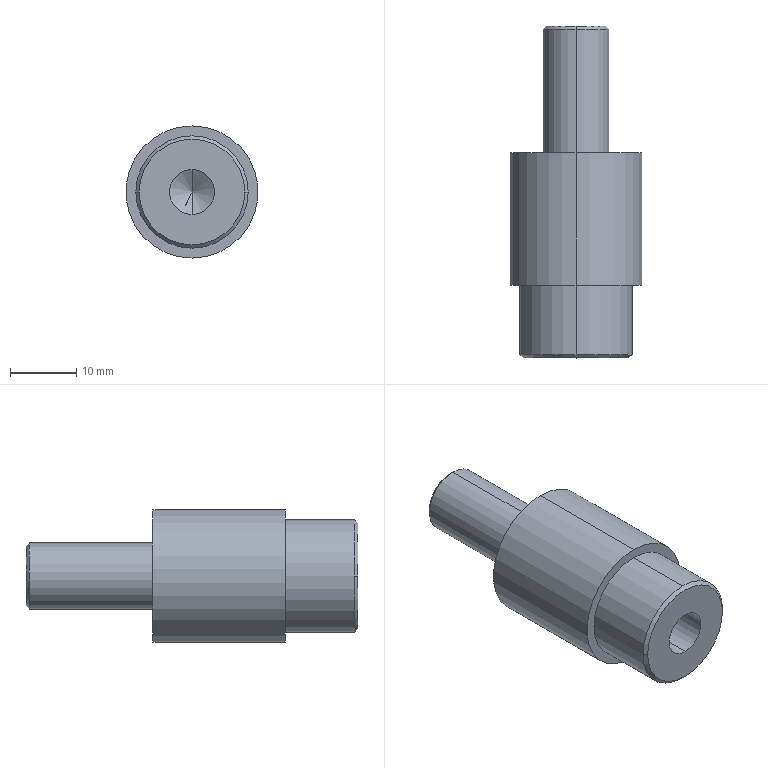Part | SolidWorks | features BaseBody 1 | 1 solid | 18 faces | box 20 x 50.2 x 20 mm | volume 9817 mm3 | cylinder 8 | cone 6 | plane 4 | commonest cylinder face diameters 6.8 x2 10 x2 17 x2 20 x2
STEP:
#1=CARTESIAN_POINT('',(0.,20.,-10.));
#2=VERTEX_POINT('',#1);
#3=CARTESIAN_POINT('',(0.,20.,10.));
#4=VERTEX_POINT('',#3);
#5=CARTESIAN_POINT('',(0.,20.,0.));
#6=DIRECTION('',(0.,-1.,0.));
#7=DIRECTION('',(0.,0.,-1.));
#8=AXIS2_PLACEMENT_3D('',#5,#6,#7);
#9=CIRCLE('',#8,10.);
#10=EDGE_CURVE('',#2,#4,#9,.T.);
#11=ORIENTED_EDGE('',*,*,#10,.T.);
#12=CARTESIAN_POINT('',(0.,0.,10.));
#13=VERTEX_POINT('',#12);
#14=CARTESIAN_POINT('',(0.,20.,10.));
#15=DIRECTION('',(0.,-1.,0.));
#16=VECTOR('',#15,1000.);
#17=LINE('',#14,#16);
#18=EDGE_CURVE('',#4,#13,#17,.T.);
#19=ORIENTED_EDGE('',*,*,#18,.T.);
#20=CARTESIAN_POINT('',(0.,0.,-10.));
#21=VERTEX_POINT('',#20);
#22=CARTESIAN_POINT('',(0.,0.,0.));
#23=DIRECTION('',(0.,1.,0.));
#24=DIRECTION('',(0.,0.,-1.));
#25=AXIS2_PLACEMENT_3D('',#22,#23,#24);
#26=CIRCLE('',#25,10.);
#27=EDGE_CURVE('',#13,#21,#26,.T.);
#28=ORIENTED_EDGE('',*,*,#27,.T.);
#29=CARTESIAN_POINT('',(0.,20.,-10.));
#30=DIRECTION('',(0.,-1.,0.));
#31=VECTOR('',#30,1000.);
#32=LINE('',#29,#31);
#33=EDGE_CURVE('',#2,#21,#32,.T.);
#34=ORIENTED_EDGE('',*,*,#33,.F.);
#35=EDGE_LOOP('',(#11,#19,#28,#34));
#36=FACE_OUTER_BOUND('',#35,.T.);
#37=CARTESIAN_POINT('',(0.,20.,0.));
#38=DIRECTION('',(0.,-1.,0.));
#39=DIRECTION('',(0.,0.,-1.));
#40=AXIS2_PLACEMENT_3D('',#37,#38,#39);
#41=CYLINDRICAL_SURFACE('',#40,10.);
#42=ADVANCED_FACE('',(#36),#41,.T.);
#43=CARTESIAN_POINT('',(8.5,-10.5,0.));
#44=VERTEX_POINT('',#43);
#45=CARTESIAN_POINT('',(0.,-10.5,-8.5));
#46=VERTEX_POINT('',#45);
#47=CARTESIAN_POINT('',(0.,-10.5,0.));
#48=DIRECTION('',(0.,1.,0.));
#49=DIRECTION('',(0.,0.,1.));
#50=AXIS2_PLACEMENT_3D('',#47,#48,#49);
#51=CIRCLE('',#50,8.5);
#52=EDGE_CURVE('',#44,#46,#51,.T.);
#53=ORIENTED_EDGE('',*,*,#52,.T.);
#54=CARTESIAN_POINT('',(0.,0.,-8.5));
#55=VERTEX_POINT('',#54);
#56=CARTESIAN_POINT('',(0.,-11.,-8.5));
#57=DIRECTION('',(0.,1.,0.));
#58=VECTOR('',#57,1000.);
#59=LINE('',#56,#58);
#60=EDGE_CURVE('',#46,#55,#59,.T.);
#61=ORIENTED_EDGE('',*,*,#60,.T.);
#62=CARTESIAN_POINT('',(0.,0.,8.5));
#63=VERTEX_POINT('',#62);
#64=CARTESIAN_POINT('',(0.,0.,0.));
#65=DIRECTION('',(0.,-1.,0.));
#66=DIRECTION('',(0.,0.,1.));
#67=AXIS2_PLACEMENT_3D('',#64,#65,#66);
#68=CIRCLE('',#67,8.5);
#69=EDGE_CURVE('',#55,#63,#68,.T.);
#70=ORIENTED_EDGE('',*,*,#69,.T.);
#71=CARTESIAN_POINT('',(0.,-10.5,8.5));
#72=VERTEX_POINT('',#71);
#73=CARTESIAN_POINT('',(0.,-11.,8.5));
#74=DIRECTION('',(0.,1.,0.));
#75=VECTOR('',#74,1000.);
#76=LINE('',#73,#75);
#77=EDGE_CURVE('',#72,#63,#76,.T.);
#78=ORIENTED_EDGE('',*,*,#77,.F.);
#79=CARTESIAN_POINT('',(0.,-10.5,0.));
#80=DIRECTION('',(0.,1.,0.));
#81=DIRECTION('',(0.,0.,1.));
#82=AXIS2_PLACEMENT_3D('',#79,#80,#81);
#83=CIRCLE('',#82,8.5);
#84=EDGE_CURVE('',#72,#44,#83,.T.);
#85=ORIENTED_EDGE('',*,*,#84,.T.);
#86=EDGE_LOOP('',(#53,#61,#70,#78,#85));
#87=FACE_OUTER_BOUND('',#86,.T.);
#88=CARTESIAN_POINT('',(0.,-11.,0.));
#89=DIRECTION('',(0.,1.,0.));
#90=DIRECTION('',(0.,0.,1.));
#91=AXIS2_PLACEMENT_3D('',#88,#89,#90);
#92=CYLINDRICAL_SURFACE('',#91,8.5);
#93=ADVANCED_FACE('',(#87),#92,.T.);
#94=CARTESIAN_POINT('',(0.,38.7,-5.));
#95=VERTEX_POINT('',#94);
#96=CARTESIAN_POINT('',(0.,38.7,5.));
#97=VERTEX_POINT('',#96);
#98=CARTESIAN_POINT('',(0.,38.7,0.));
#99=DIRECTION('',(0.,-1.,0.));
#100=DIRECTION('',(0.,0.,-1.));
#101=AXIS2_PLACEMENT_3D('',#98,#99,#100);
#102=CIRCLE('',#101,5.);
#103=EDGE_CURVE('',#95,#97,#102,.T.);
#104=ORIENTED_EDGE('',*,*,#103,.T.);
#105=CARTESIAN_POINT('',(0.,20.,5.));
#106=VERTEX_POINT('',#105);
#107=CARTESIAN_POINT('',(0.,39.2,5.));
#108=DIRECTION('',(0.,-1.,0.));
#109=VECTOR('',#108,1000.);
#110=LINE('',#107,#109);
#111=EDGE_CURVE('',#97,#106,#110,.T.);
#112=ORIENTED_EDGE('',*,*,#111,.T.);
#113=CARTESIAN_POINT('',(0.,20.,-5.));
#114=VERTEX_POINT('',#113);
#115=CARTESIAN_POINT('',(0.,20.,0.));
#116=DIRECTION('',(0.,-1.,0.));
#117=DIRECTION('',(0.,0.,-1.));
#118=AXIS2_PLACEMENT_3D('',#115,#116,#117);
#119=CIRCLE('',#118,5.);
#120=EDGE_CURVE('',#114,#106,#119,.T.);
#121=ORIENTED_EDGE('',*,*,#120,.F.);
#122=CARTESIAN_POINT('',(0.,39.2,-5.));
#123=DIRECTION('',(0.,-1.,0.));
#124=VECTOR('',#123,1000.);
#125=LINE('',#122,#124);
#126=EDGE_CURVE('',#95,#114,#125,.T.);
#127=ORIENTED_EDGE('',*,*,#126,.F.);
#128=EDGE_LOOP('',(#104,#112,#121,#127));
#129=FACE_OUTER_BOUND('',#128,.T.);
#130=CARTESIAN_POINT('',(0.,39.2,0.));
#131=DIRECTION('',(0.,-1.,0.));
#132=DIRECTION('',(0.,0.,-1.));
#133=AXIS2_PLACEMENT_3D('',#130,#131,#132);
#134=CYLINDRICAL_SURFACE('',#133,5.);
#135=ADVANCED_FACE('',(#129),#134,.T.);
#136=CARTESIAN_POINT('',(-8.,-11.,0.));
#137=VERTEX_POINT('',#136);
#138=CARTESIAN_POINT('',(8.,-11.,0.));
#139=VERTEX_POINT('',#138);
#140=CARTESIAN_POINT('',(0.,-11.,0.));
#141=DIRECTION('',(0.,1.,0.));
#142=DIRECTION('',(-1.,0.,0.));
#143=AXIS2_PLACEMENT_3D('',#140,#141,#142);
#144=CIRCLE('',#143,8.);
#145=EDGE_CURVE('',#137,#139,#144,.T.);
#146=ORIENTED_EDGE('',*,*,#145,.T.);
#147=CARTESIAN_POINT('',(8.5,-10.5,0.));
#148=DIRECTION('',(0.7071,0.7071,0.));
#149=VECTOR('',#148,1000.);
#150=LINE('',#147,#149);
#151=EDGE_CURVE('',#139,#44,#150,.T.);
#152=ORIENTED_EDGE('',*,*,#151,.T.);
#153=ORIENTED_EDGE('',*,*,#84,.F.);
#154=CARTESIAN_POINT('',(-8.5,-10.5,0.));
#155=VERTEX_POINT('',#154);
#156=CARTESIAN_POINT('',(0.,-10.5,0.));
#157=DIRECTION('',(0.,1.,0.));
#158=DIRECTION('',(0.,0.,1.));
#159=AXIS2_PLACEMENT_3D('',#156,#157,#158);
#160=CIRCLE('',#159,8.5);
#161=EDGE_CURVE('',#155,#72,#160,.T.);
#162=ORIENTED_EDGE('',*,*,#161,.F.);
#163=CARTESIAN_POINT('',(-8.5,-10.5,0.));
#164=DIRECTION('',(-0.7071,0.7071,0.));
#165=VECTOR('',#164,1000.);
#166=LINE('',#163,#165);
#167=EDGE_CURVE('',#137,#155,#166,.T.);
#168=ORIENTED_EDGE('',*,*,#167,.F.);
#169=EDGE_LOOP('',(#146,#152,#153,#162,#168));
#170=FACE_OUTER_BOUND('',#169,.T.);
#171=CARTESIAN_POINT('',(0.,-10.5,0.));
#172=DIRECTION('',(0.,1.,0.));
#173=DIRECTION('',(-1.,0.,0.));
#174=AXIS2_PLACEMENT_3D('',#171,#172,#173);
#175=CONICAL_SURFACE('',#174,8.5,0.7854);
#176=ADVANCED_FACE('',(#170),#175,.T.);
#177=CARTESIAN_POINT('',(0.,39.2,-4.5));
#178=VERTEX_POINT('',#177);
#179=CARTESIAN_POINT('',(0.,39.2,4.5));
#180=VERTEX_POINT('',#179);
#181=CARTESIAN_POINT('',(0.,39.2,0.));
#182=DIRECTION('',(0.,-1.,0.));
#183=DIRECTION('',(0.,0.,-1.));
#184=AXIS2_PLACEMENT_3D('',#181,#182,#183);
#185=CIRCLE('',#184,4.5);
#186=EDGE_CURVE('',#178,#180,#185,.T.);
#187=ORIENTED_EDGE('',*,*,#186,.T.);
#188=CARTESIAN_POINT('',(0.,38.7,5.));
#189=DIRECTION('',(0.,-0.7071,0.7071));
#190=VECTOR('',#189,1000.);
#191=LINE('',#188,#190);
#192=EDGE_CURVE('',#180,#97,#191,.T.);
#193=ORIENTED_EDGE('',*,*,#192,.T.);
#194=ORIENTED_EDGE('',*,*,#103,.F.);
#195=CARTESIAN_POINT('',(0.,38.7,-5.));
#196=DIRECTION('',(0.,-0.7071,-0.7071));
#197=VECTOR('',#196,1000.);
#198=LINE('',#195,#197);
#199=EDGE_CURVE('',#178,#95,#198,.T.);
#200=ORIENTED_EDGE('',*,*,#199,.F.);
#201=EDGE_LOOP('',(#187,#193,#194,#200));
#202=FACE_OUTER_BOUND('',#201,.T.);
#203=CARTESIAN_POINT('',(0.,38.7,0.));
#204=DIRECTION('',(0.,-1.,0.));
#205=DIRECTION('',(0.,0.,-1.));
#206=AXIS2_PLACEMENT_3D('',#203,#204,#205);
#207=CONICAL_SURFACE('',#206,5.,0.7854);
#208=ADVANCED_FACE('',(#202),#207,.T.);
#209=CARTESIAN_POINT('',(0.,1.,3.4));
#210=VERTEX_POINT('',#209);
#211=CARTESIAN_POINT('',(0.,1.,-3.4));
#212=VERTEX_POINT('',#211);
#213=CARTESIAN_POINT('',(0.,1.,0.));
#214=DIRECTION('',(0.,-1.,0.));
#215=DIRECTION('',(0.,0.,-1.));
#216=AXIS2_PLACEMENT_3D('',#213,#214,#215);
#217=CIRCLE('',#216,3.4);
#218=EDGE_CURVE('',#210,#212,#217,.T.);
#219=ORIENTED_EDGE('',*,*,#218,.F.);
#220=CARTESIAN_POINT('',(0.,-11.,3.4));
#221=VERTEX_POINT('',#220);
#222=CARTESIAN_POINT('',(0.,-11.,3.4));
#223=DIRECTION('',(0.,-1.,0.));
#224=VECTOR('',#223,1000.);
#225=LINE('',#222,#224);
#226=EDGE_CURVE('',#210,#221,#225,.T.);
#227=ORIENTED_EDGE('',*,*,#226,.T.);
#228=CARTESIAN_POINT('',(0.,-11.,-3.4));
#229=VERTEX_POINT('',#228);
#230=CARTESIAN_POINT('',(0.,-11.,0.));
#231=DIRECTION('',(0.,1.,0.));
#232=DIRECTION('',(0.,0.,-1.));
#233=AXIS2_PLACEMENT_3D('',#230,#231,#232);
#234=CIRCLE('',#233,3.4);
#235=EDGE_CURVE('',#229,#221,#234,.T.);
#236=ORIENTED_EDGE('',*,*,#235,.F.);
#237=CARTESIAN_POINT('',(0.,-11.,-3.4));
#238=DIRECTION('',(0.,-1.,0.));
#239=VECTOR('',#238,1000.);
#240=LINE('',#237,#239);
#241=EDGE_CURVE('',#212,#229,#240,.T.);
#242=ORIENTED_EDGE('',*,*,#241,.F.);
#243=EDGE_LOOP('',(#219,#227,#236,#242));
#244=FACE_OUTER_BOUND('',#243,.T.);
#245=CARTESIAN_POINT('',(0.,-11.,0.));
#246=DIRECTION('',(0.,-1.,0.));
#247=DIRECTION('',(0.,0.,-1.));
#248=AXIS2_PLACEMENT_3D('',#245,#246,#247);
#249=CYLINDRICAL_SURFACE('',#248,3.4);
#250=ADVANCED_FACE('',(#244),#249,.F.);
#251=CARTESIAN_POINT('',(0.,3.043,0.));
#252=VERTEX_POINT('',#251);
#253=CARTESIAN_POINT('',(0.,1.,-3.4));
#254=DIRECTION('',(0.,-0.515,-0.8572));
#255=VECTOR('',#254,1000.);
#256=LINE('',#253,#255);
#257=EDGE_CURVE('',#252,#212,#256,.T.);
#258=ORIENTED_EDGE('',*,*,#257,.F.);
#259=CARTESIAN_POINT('',(0.,1.,3.4));
#260=DIRECTION('',(0.,-0.515,0.8572));
#261=VECTOR('',#260,1000.);
#262=LINE('',#259,#261);
#263=EDGE_CURVE('',#252,#210,#262,.T.);
#264=ORIENTED_EDGE('',*,*,#263,.T.);
#265=ORIENTED_EDGE('',*,*,#218,.T.);
#266=EDGE_LOOP('',(#258,#264,#265));
#267=FACE_OUTER_BOUND('',#266,.T.);
#268=CARTESIAN_POINT('',(0.,1.,0.));
#269=DIRECTION('',(0.,-1.,0.));
#270=DIRECTION('',(0.,0.,-1.));
#271=AXIS2_PLACEMENT_3D('',#268,#269,#270);
#272=CONICAL_SURFACE('',#271,3.4,1.03);
#273=ADVANCED_FACE('',(#267),#272,.F.);
#274=ORIENTED_EDGE('',*,*,#18,.F.);
#275=CARTESIAN_POINT('',(0.,20.,0.));
#276=DIRECTION('',(0.,-1.,0.));
#277=DIRECTION('',(0.,0.,-1.));
#278=AXIS2_PLACEMENT_3D('',#275,#276,#277);
#279=CIRCLE('',#278,10.);
#280=EDGE_CURVE('',#4,#2,#279,.T.);
#281=ORIENTED_EDGE('',*,*,#280,.T.);
#282=ORIENTED_EDGE('',*,*,#33,.T.);
#283=CARTESIAN_POINT('',(0.,0.,0.));
#284=DIRECTION('',(0.,1.,0.));
#285=DIRECTION('',(0.,0.,-1.));
#286=AXIS2_PLACEMENT_3D('',#283,#284,#285);
#287=CIRCLE('',#286,10.);
#288=EDGE_CURVE('',#21,#13,#287,.T.);
#289=ORIENTED_EDGE('',*,*,#288,.T.);
#290=EDGE_LOOP('',(#274,#281,#282,#289));
#291=FACE_OUTER_BOUND('',#290,.T.);
#292=CARTESIAN_POINT('',(0.,20.,0.));
#293=DIRECTION('',(0.,-1.,0.));
#294=DIRECTION('',(0.,0.,-1.));
#295=AXIS2_PLACEMENT_3D('',#292,#293,#294);
#296=CYLINDRICAL_SURFACE('',#295,10.);
#297=ADVANCED_FACE('',(#291),#296,.T.);
#298=ORIENTED_EDGE('',*,*,#288,.F.);
#299=ORIENTED_EDGE('',*,*,#27,.F.);
#300=EDGE_LOOP('',(#298,#299));
#301=FACE_OUTER_BOUND('',#300,.T.);
#302=CARTESIAN_POINT('',(0.,0.,0.));
#303=DIRECTION('',(0.,-1.,0.));
#304=DIRECTION('',(0.,0.,1.));
#305=AXIS2_PLACEMENT_3D('',#302,#303,#304);
#306=CIRCLE('',#305,8.5);
#307=EDGE_CURVE('',#63,#55,#306,.T.);
#308=ORIENTED_EDGE('',*,*,#307,.F.);
#309=ORIENTED_EDGE('',*,*,#69,.F.);
#310=EDGE_LOOP('',(#308,#309));
#311=FACE_BOUND('',#310,.T.);
#312=CARTESIAN_POINT('',(0.,0.,0.));
#313=DIRECTION('',(0.,1.,0.));
#314=DIRECTION('',(0.,0.,1.));
#315=AXIS2_PLACEMENT_3D('',#312,#313,#314);
#316=PLANE('',#315);
#317=ADVANCED_FACE('',(#301,#311),#316,.F.);
#318=ORIENTED_EDGE('',*,*,#10,.F.);
#319=ORIENTED_EDGE('',*,*,#280,.F.);
#320=EDGE_LOOP('',(#318,#319));
#321=FACE_OUTER_BOUND('',#320,.T.);
#322=ORIENTED_EDGE('',*,*,#120,.T.);
#323=CARTESIAN_POINT('',(0.,20.,0.));
#324=DIRECTION('',(0.,-1.,0.));
#325=DIRECTION('',(0.,0.,-1.));
#326=AXIS2_PLACEMENT_3D('',#323,#324,#325);
#327=CIRCLE('',#326,5.);
#328=EDGE_CURVE('',#106,#114,#327,.T.);
#329=ORIENTED_EDGE('',*,*,#328,.T.);
#330=EDGE_LOOP('',(#322,#329));
#331=FACE_BOUND('',#330,.T.);
#332=CARTESIAN_POINT('',(0.,20.,0.));
#333=DIRECTION('',(0.,1.,0.));
#334=DIRECTION('',(0.,0.,1.));
#335=AXIS2_PLACEMENT_3D('',#332,#333,#334);
#336=PLANE('',#335);
#337=ADVANCED_FACE('',(#321,#331),#336,.T.);
#338=ORIENTED_EDGE('',*,*,#60,.F.);
#339=CARTESIAN_POINT('',(0.,-10.5,0.));
#340=DIRECTION('',(0.,1.,0.));
#341=DIRECTION('',(0.,0.,1.));
#342=AXIS2_PLACEMENT_3D('',#339,#340,#341);
#343=CIRCLE('',#342,8.5);
#344=EDGE_CURVE('',#46,#155,#343,.T.);
#345=ORIENTED_EDGE('',*,*,#344,.T.);
#346=ORIENTED_EDGE('',*,*,#161,.T.);
#347=ORIENTED_EDGE('',*,*,#77,.T.);
#348=ORIENTED_EDGE('',*,*,#307,.T.);
#349=EDGE_LOOP('',(#338,#345,#346,#347,#348));
#350=FACE_OUTER_BOUND('',#349,.T.);
#351=CARTESIAN_POINT('',(0.,-11.,0.));
#352=DIRECTION('',(0.,1.,0.));
#353=DIRECTION('',(0.,0.,1.));
#354=AXIS2_PLACEMENT_3D('',#351,#352,#353);
#355=CYLINDRICAL_SURFACE('',#354,8.5);
#356=ADVANCED_FACE('',(#350),#355,.T.);
#357=ORIENTED_EDGE('',*,*,#111,.F.);
#358=CARTESIAN_POINT('',(0.,38.7,0.));
#359=DIRECTION('',(0.,-1.,0.));
#360=DIRECTION('',(0.,0.,-1.));
#361=AXIS2_PLACEMENT_3D('',#358,#359,#360);
#362=CIRCLE('',#361,5.);
#363=EDGE_CURVE('',#97,#95,#362,.T.);
#364=ORIENTED_EDGE('',*,*,#363,.T.);
#365=ORIENTED_EDGE('',*,*,#126,.T.);
#366=ORIENTED_EDGE('',*,*,#328,.F.);
#367=EDGE_LOOP('',(#357,#364,#365,#366));
#368=FACE_OUTER_BOUND('',#367,.T.);
#369=CARTESIAN_POINT('',(0.,39.2,0.));
#370=DIRECTION('',(0.,-1.,0.));
#371=DIRECTION('',(0.,0.,-1.));
#372=AXIS2_PLACEMENT_3D('',#369,#370,#371);
#373=CYLINDRICAL_SURFACE('',#372,5.);
#374=ADVANCED_FACE('',(#368),#373,.T.);
#375=ORIENTED_EDGE('',*,*,#151,.F.);
#376=CARTESIAN_POINT('',(0.,-11.,0.));
#377=DIRECTION('',(0.,1.,0.));
#378=DIRECTION('',(-1.,0.,0.));
#379=AXIS2_PLACEMENT_3D('',#376,#377,#378);
#380=CIRCLE('',#379,8.);
#381=EDGE_CURVE('',#139,#137,#380,.T.);
#382=ORIENTED_EDGE('',*,*,#381,.T.);
#383=ORIENTED_EDGE('',*,*,#167,.T.);
#384=ORIENTED_EDGE('',*,*,#344,.F.);
#385=ORIENTED_EDGE('',*,*,#52,.F.);
#386=EDGE_LOOP('',(#375,#382,#383,#384,#385));
#387=FACE_OUTER_BOUND('',#386,.T.);
#388=CARTESIAN_POINT('',(0.,-10.5,0.));
#389=DIRECTION('',(0.,1.,0.));
#390=DIRECTION('',(-1.,0.,0.));
#391=AXIS2_PLACEMENT_3D('',#388,#389,#390);
#392=CONICAL_SURFACE('',#391,8.5,0.7854);
#393=ADVANCED_FACE('',(#387),#392,.T.);
#394=ORIENTED_EDGE('',*,*,#192,.F.);
#395=CARTESIAN_POINT('',(0.,39.2,0.));
#396=DIRECTION('',(0.,-1.,0.));
#397=DIRECTION('',(0.,0.,-1.));
#398=AXIS2_PLACEMENT_3D('',#395,#396,#397);
#399=CIRCLE('',#398,4.5);
#400=EDGE_CURVE('',#180,#178,#399,.T.);
#401=ORIENTED_EDGE('',*,*,#400,.T.);
#402=ORIENTED_EDGE('',*,*,#199,.T.);
#403=ORIENTED_EDGE('',*,*,#363,.F.);
#404=EDGE_LOOP('',(#394,#401,#402,#403));
#405=FACE_OUTER_BOUND('',#404,.T.);
#406=CARTESIAN_POINT('',(0.,38.7,0.));
#407=DIRECTION('',(0.,-1.,0.));
#408=DIRECTION('',(0.,0.,-1.));
#409=AXIS2_PLACEMENT_3D('',#406,#407,#408);
#410=CONICAL_SURFACE('',#409,5.,0.7854);
#411=ADVANCED_FACE('',(#405),#410,.T.);
#412=ORIENTED_EDGE('',*,*,#235,.T.);
#413=CARTESIAN_POINT('',(0.,-11.,0.));
#414=DIRECTION('',(0.,1.,0.));
#415=DIRECTION('',(0.,0.,-1.));
#416=AXIS2_PLACEMENT_3D('',#413,#414,#415);
#417=CIRCLE('',#416,3.4);
#418=EDGE_CURVE('',#221,#229,#417,.T.);
#419=ORIENTED_EDGE('',*,*,#418,.T.);
#420=EDGE_LOOP('',(#412,#419));
#421=FACE_BOUND('',#420,.T.);
#422=ORIENTED_EDGE('',*,*,#145,.F.);
#423=ORIENTED_EDGE('',*,*,#381,.F.);
#424=EDGE_LOOP('',(#422,#423));
#425=FACE_OUTER_BOUND('',#424,.T.);
#426=CARTESIAN_POINT('',(0.,-11.,0.));
#427=DIRECTION('',(0.,-1.,0.));
#428=DIRECTION('',(0.,0.,-1.));
#429=AXIS2_PLACEMENT_3D('',#426,#427,#428);
#430=PLANE('',#429);
#431=ADVANCED_FACE('',(#421,#425),#430,.T.);
#432=ORIENTED_EDGE('',*,*,#186,.F.);
#433=ORIENTED_EDGE('',*,*,#400,.F.);
#434=EDGE_LOOP('',(#432,#433));
#435=FACE_OUTER_BOUND('',#434,.T.);
#436=CARTESIAN_POINT('',(0.,39.2,0.));
#437=DIRECTION('',(0.,1.,0.));
#438=DIRECTION('',(0.,0.,1.));
#439=AXIS2_PLACEMENT_3D('',#436,#437,#438);
#440=PLANE('',#439);
#441=ADVANCED_FACE('',(#435),#440,.T.);
#442=ORIENTED_EDGE('',*,*,#226,.F.);
#443=CARTESIAN_POINT('',(0.,1.,0.));
#444=DIRECTION('',(0.,-1.,0.));
#445=DIRECTION('',(0.,0.,-1.));
#446=AXIS2_PLACEMENT_3D('',#443,#444,#445);
#447=CIRCLE('',#446,3.4);
#448=EDGE_CURVE('',#212,#210,#447,.T.);
#449=ORIENTED_EDGE('',*,*,#448,.F.);
#450=ORIENTED_EDGE('',*,*,#241,.T.);
#451=ORIENTED_EDGE('',*,*,#418,.F.);
#452=EDGE_LOOP('',(#442,#449,#450,#451));
#453=FACE_OUTER_BOUND('',#452,.T.);
#454=CARTESIAN_POINT('',(0.,-11.,0.));
#455=DIRECTION('',(0.,-1.,0.));
#456=DIRECTION('',(0.,0.,-1.));
#457=AXIS2_PLACEMENT_3D('',#454,#455,#456);
#458=CYLINDRICAL_SURFACE('',#457,3.4);
#459=ADVANCED_FACE('',(#453),#458,.F.);
#460=ORIENTED_EDGE('',*,*,#263,.F.);
#461=ORIENTED_EDGE('',*,*,#257,.T.);
#462=ORIENTED_EDGE('',*,*,#448,.T.);
#463=EDGE_LOOP('',(#460,#461,#462));
#464=FACE_OUTER_BOUND('',#463,.T.);
#465=CARTESIAN_POINT('',(0.,1.,0.));
#466=DIRECTION('',(0.,-1.,0.));
#467=DIRECTION('',(0.,0.,-1.));
#468=AXIS2_PLACEMENT_3D('',#465,#466,#467);
#469=CONICAL_SURFACE('',#468,3.4,1.03);
#470=ADVANCED_FACE('',(#464),#469,.F.);
#471=CLOSED_SHELL('',(#42,#93,#135,#176,#208,#250,#273,#297,#317,#337,#356,#374,#393,#411,#431,#441,#459,#470));
#472=MANIFOLD_SOLID_BREP('',#471);
#473=CARTESIAN_POINT('',(0.,0.,0.));
#474=DIRECTION('',(0.,0.,1.));
#475=DIRECTION('',(1.,0.,0.));
#476=AXIS2_PLACEMENT_3D('',#473,#474,#475);
#477=(LENGTH_UNIT()NAMED_UNIT(*)SI_UNIT(.MILLI.,.METRE.));
#478=UNCERTAINTY_MEASURE_WITH_UNIT(LENGTH_MEASURE(0.00001),#477,'','');
#479=(NAMED_UNIT(*)PLANE_ANGLE_UNIT()SI_UNIT($,.RADIAN.));
#480=(NAMED_UNIT(*)SI_UNIT($,.STERADIAN.)SOLID_ANGLE_UNIT());
#481=(GEOMETRIC_REPRESENTATION_CONTEXT(3)GLOBAL_UNCERTAINTY_ASSIGNED_CONTEXT((#478))GLOBAL_UNIT_ASSIGNED_CONTEXT((#477,#479,#480))REPRESENTATION_CONTEXT('',''));
#482=ADVANCED_BREP_SHAPE_REPRESENTATION('',(#472,#476),#481);